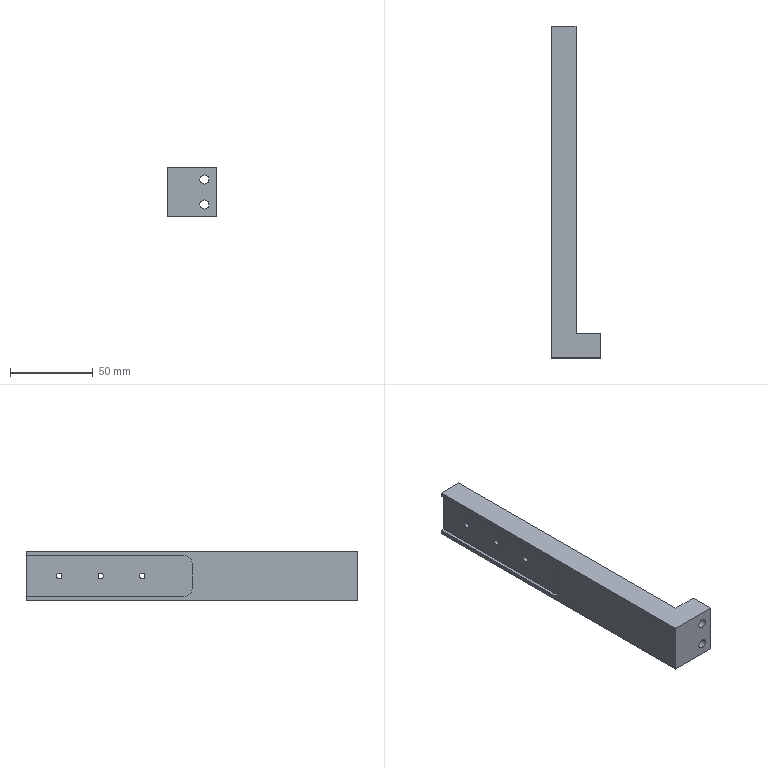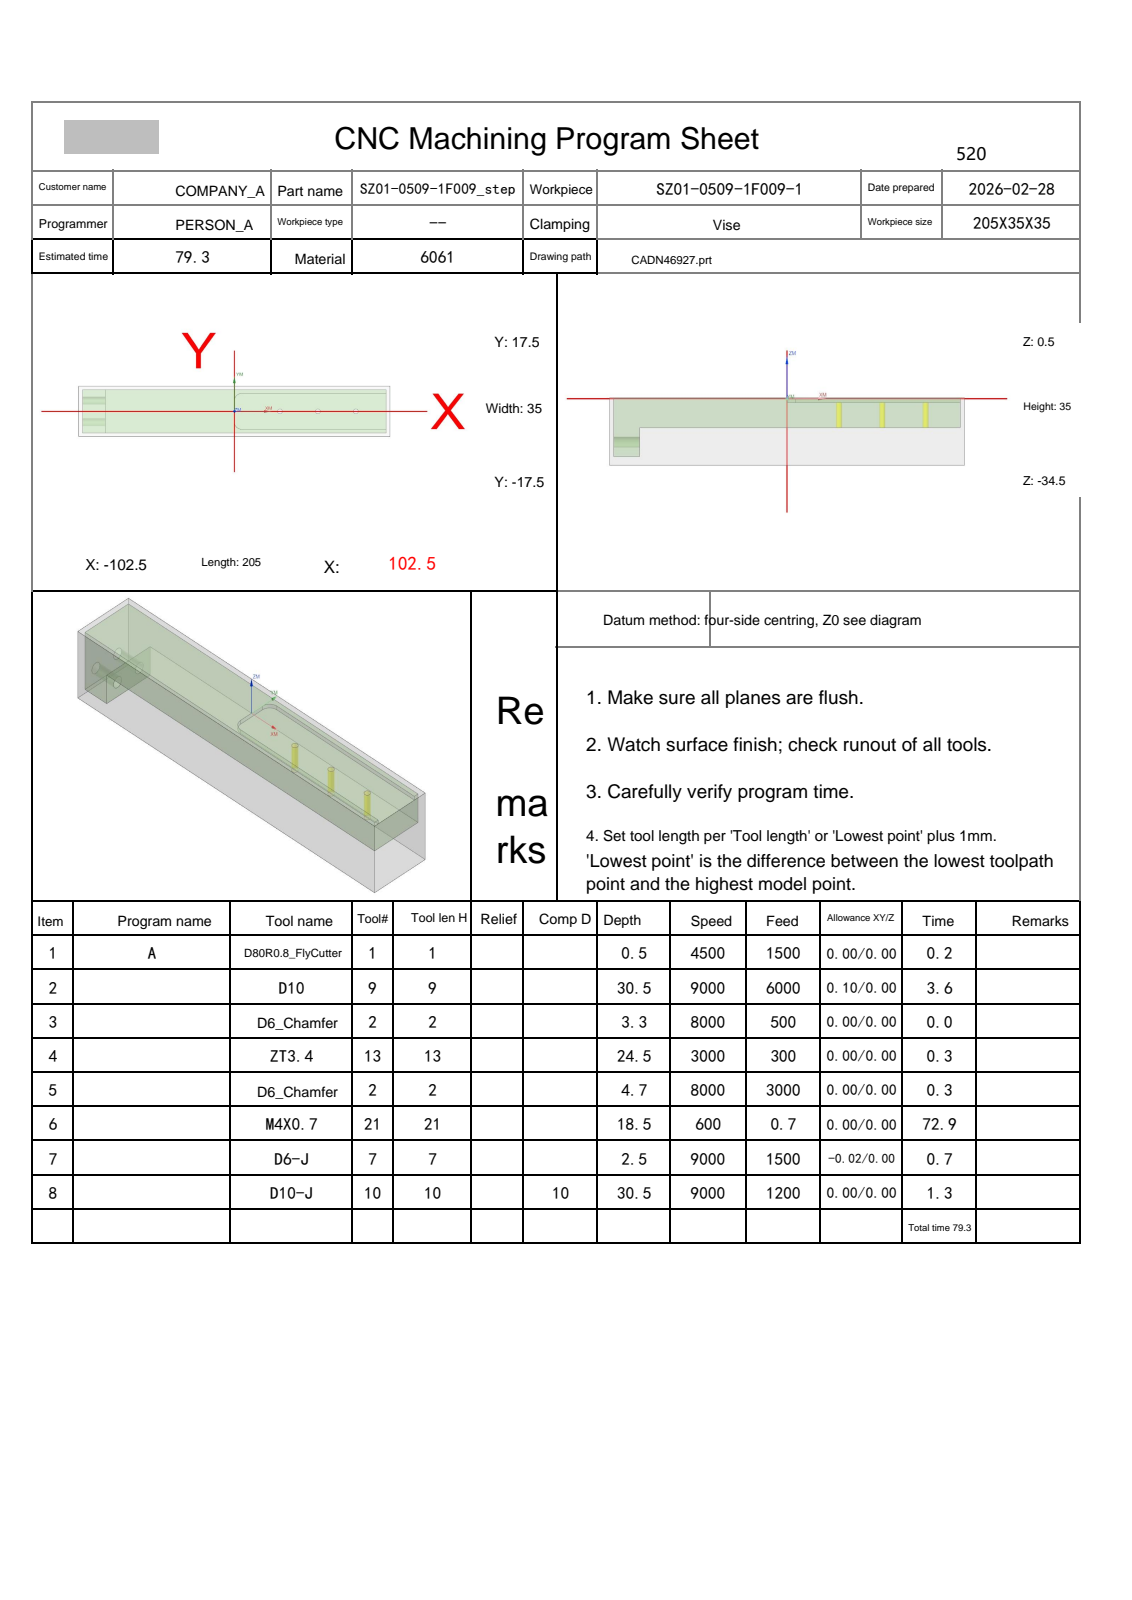NC program | NX | posted by the shop | part box 30 x 200 x 30 mm
Whole program:
%
O0001
(Machine time: 149.40 MIN)
(===Total Tool:7===)
(T1=D80R0.8-FlyCutter D=80.  R=0.8  D-  H01 Z=0.    )
(T9=D10     D=10.  R=0.   D-  H09 Z=-30.  )
(T2=D6_Chamfer   D=6.   R=0.   D-  H02 Z=-4.2  )
(T13=ZT3.4  D=3.4  DR_a=118 D-  H13 Z=-24.  )
(T21=M4X0.7 D=3.3  DR_a=180 D-  H21 Z=-18.  )
(T7=D6-J    D=6.   R=0.   D7  H07 Z=-2.   )
(T10=D10-J  D=10.  R=0.   D10 H10 Z=-30.  )
G80 G90 G17 G49 G40
G91 G28 Z0
M01
N1 T01 M06
(D80R0.8-FlyCutter  D=80. R=0.8 H=01 ce=0.00 di=0.00)
G00 G90 G54 X-145. Y0.0 M03 S4500
G43 H01 Z50.
M08
Z2.
G01 Z0.0 F1500.
X-140.
X140.
X145.
Z2.
G00 Z50.
G91 G28 Z0.0
M05
M09
G91 G28 Z0.0
M01
N2 T09 M06
(D10  D=10. R=0. H=09 ce=0.10 di=0.00)
G00 G90 G54 X0.0 Y20.1 M03 S8000
G43 H09 Z50.
M08
Z.5
G01 X100. Z.341 F6000.
G02 X105.1 Y15. Z.328 I0.0 J-5.1
G01 Y-15. Z.281
G02 X100. Y-20.1 Z.268 I-5.1 J0.0
G01 X-100. Z-.05
G02 X-105.1 Y-15. Z-.063 I0.0 J5.1
G01 Y15. Z-.11
G02 X-100. Y20.1 Z-.123 I5.1 J0.0
G01 X100. Z-.441
G02 X105.1 Y15. Z-.454 I0.0 J-5.1
G01 Y-15. Z-.501
G02 X100. Y-20.1 Z-.514 I-5.1 J0.0
G01 X-100. Z-.832
G02 X-105.1 Y-15. Z-.845 I0.0 J5.1
G01 Y15. Z-.892
G02 X-100. Y20.1 Z-.905 I5.1 J0.0
G01 X100. Z-1.223
G02 X105.1 Y15. Z-1.236 I0.0 J-5.1
G01 Y-15. Z-1.283
G02 X100. Y-20.1 Z-1.296 I-5.1 J0.0
G01 X-100. Z-1.614
G02 X-105.1 Y-15. Z-1.627 I0.0 J5.1
G01 Y15. Z-1.674
G02 X-100. Y20.1 Z-1.687 I5.1 J0.0
G01 X100. Z-2.005
G02 X105.1 Y15. Z-2.018 I0.0 J-5.1
G01 Y-15. Z-2.066
G02 X100. Y-20.1 Z-2.078 I-5.1 J0.0
G01 X-100. Z-2.396
G02 X-105.1 Y-15. Z-2.409 I0.0 J5.1
G01 Y15. Z-2.457
G02 X-100. Y20.1 Z-2.469 I5.1 J0.0
G01 X100. Z-2.787
G02 X105.1 Y15. Z-2.8 I0.0 J-5.1
G01 Y-15. Z-2.848
G02 X100. Y-20.1 Z-2.86 I-5.1 J0.0
G01 X-100. Z-3.178
G02 X-105.1 Y-15. Z-3.191 I0.0 J5.1
G01 Y15. Z-3.239
G02 X-100. Y20.1 Z-3.251 I5.1 J0.0
G01 X100. Z-3.569
G02 X105.1 Y15. Z-3.582 I0.0 J-5.1
G01 Y-15. Z-3.63
G02 X100. Y-20.1 Z-3.642 I-5.1 J0.0
G01 X-100. Z-3.96
G02 X-105.1 Y-15. Z-3.973 I0.0 J5.1
G01 Y15. Z-4.021
G02 X-100. Y20.1 Z-4.033 I5.1 J0.0
G01 X100. Z-4.351
G02 X105.1 Y15. Z-4.364 I0.0 J-5.1
G01 Y-15. Z-4.412
G02 X100. Y-20.1 Z-4.424 I-5.1 J0.0
G01 X-100. Z-4.742
G02 X-105.1 Y-15. Z-4.755 I0.0 J5.1
G01 Y15. Z-4.803
G02 X-100. Y20.1 Z-4.815 I5.1 J0.0
G01 X100. Z-5.133
G02 X105.1 Y15. Z-5.146 I0.0 J-5.1
G01 Y-15. Z-5.194
G02 X100. Y-20.1 Z-5.206 I-5.1 J0.0
G01 X-100. Z-5.524
G02 X-105.1 Y-15. Z-5.537 I0.0 J5.1
G01 Y15. Z-5.585
G02 X-100. Y20.1 Z-5.597 I5.1 J0.0
G01 X100. Z-5.915
G02 X105.1 Y15. Z-5.928 I0.0 J-5.1
G01 Y-15. Z-5.976
G02 X100. Y-20.1 Z-5.988 I-5.1 J0.0
G01 X-100. Z-6.306
G02 X-105.1 Y-15. Z-6.319 I0.0 J5.1
G01 Y15. Z-6.367
G02 X-100. Y20.1 Z-6.38 I5.1 J0.0
G01 X100. Z-6.697
G02 X105.1 Y15. Z-6.71 I0.0 J-5.1
G01 Y-15. Z-6.758
G02 X100. Y-20.1 Z-6.771 I-5.1 J0.0
G01 X-100. Z-7.088
G02 X-105.1 Y-15. Z-7.101 I0.0 J5.1
G01 Y15. Z-7.149
G02 X-100. Y20.1 Z-7.162 I5.1 J0.0
G01 X100. Z-7.479
G02 X105.1 Y15. Z-7.492 I0.0 J-5.1
G01 Y-15. Z-7.54
G02 X100. Y-20.1 Z-7.553 I-5.1 J0.0
G01 X-100. Z-7.87
G02 X-105.1 Y-15. Z-7.883 I0.0 J5.1
G01 Y15. Z-7.931
G02 X-100. Y20.1 Z-7.944 I5.1 J0.0
G01 X100. Z-8.262
G02 X105.1 Y15. Z-8.274 I0.0 J-5.1
G01 Y-15. Z-8.322
G02 X100. Y-20.1 Z-8.335 I-5.1 J0.0
G01 X-100. Z-8.653
G02 X-105.1 Y-15. Z-8.665 I0.0 J5.1
G01 Y15. Z-8.713
G02 X-100. Y20.1 Z-8.726 I5.1 J0.0
G01 X100. Z-9.044
G02 X105.1 Y15. Z-9.056 I0.0 J-5.1
G01 Y-15. Z-9.104
G02 X100. Y-20.1 Z-9.117 I-5.1 J0.0
G01 X-100. Z-9.435
G02 X-105.1 Y-15. Z-9.447 I0.0 J5.1
G01 Y15. Z-9.495
G02 X-100. Y20.1 Z-9.508 I5.1 J0.0
G01 X100. Z-9.826
G02 X105.1 Y15. Z-9.838 I0.0 J-5.1
G01 Y-15. Z-9.886
G02 X100. Y-20.1 Z-9.899 I-5.1 J0.0
G01 X-100. Z-10.217
G02 X-105.1 Y-15. Z-10.229 I0.0 J5.1
G01 Y15. Z-10.277
G02 X-100. Y20.1 Z-10.29 I5.1 J0.0
G01 X100. Z-10.608
G02 X105.1 Y15. Z-10.62 I0.0 J-5.1
G01 Y-15. Z-10.668
G02 X100. Y-20.1 Z-10.681 I-5.1 J0.0
G01 X-100. Z-10.999
G02 X-105.1 Y-15. Z-11.011 I0.0 J5.1
G01 Y15. Z-11.059
G02 X-100. Y20.1 Z-11.072 I5.1 J0.0
G01 X100. Z-11.39
G02 X105.1 Y15. Z-11.402 I0.0 J-5.1
G01 Y-15. Z-11.45
G02 X100. Y-20.1 Z-11.463 I-5.1 J0.0
G01 X-100. Z-11.781
G02 X-105.1 Y-15. Z-11.793 I0.0 J5.1
G01 Y15. Z-11.841
G02 X-100. Y20.1 Z-11.854 I5.1 J0.0
G01 X100. Z-12.172
G02 X105.1 Y15. Z-12.184 I0.0 J-5.1
G01 Y-15. Z-12.232
G02 X100. Y-20.1 Z-12.245 I-5.1 J0.0
G01 X-100. Z-12.563
G02 X-105.1 Y-15. Z-12.576 I0.0 J5.1
G01 Y15. Z-12.623
G02 X-100. Y20.1 Z-12.636 I5.1 J0.0
G01 X100. Z-12.954
G02 X105.1 Y15. Z-12.967 I0.0 J-5.1
G01 Y-15. Z-13.014
G02 X100. Y-20.1 Z-13.027 I-5.1 J0.0
G01 X-100. Z-13.345
G02 X-105.1 Y-15. Z-13.358 I0.0 J5.1
G01 Y15. Z-13.405
G02 X-100. Y20.1 Z-13.418 I5.1 J0.0
G01 X100. Z-13.736
G02 X105.1 Y15. Z-13.749 I0.0 J-5.1
G01 Y-15. Z-13.796
G02 X100. Y-20.1 Z-13.809 I-5.1 J0.0
G01 X-100. Z-14.127
G02 X-105.1 Y-15. Z-14.14 I0.0 J5.1
G01 Y15. Z-14.187
G02 X-100. Y20.1 Z-14.2 I5.1 J0.0
G01 X100. Z-14.518
G02 X105.1 Y15. Z-14.531 I0.0 J-5.1
G01 Y-15. Z-14.578
G02 X100. Y-20.1 Z-14.591 I-5.1 J0.0
G01 X-100. Z-14.909
G02 X-105.1 Y-15. Z-14.922 I0.0 J5.1
G01 Y15. Z-14.969
G02 X-100. Y20.1 Z-14.982 I5.1 J0.0
G01 X100. Z-15.3
G02 X105.1 Y15. Z-15.313 I0.0 J-5.1
G01 Y-15. Z-15.36
G02 X100. Y-20.1 Z-15.373 I-5.1 J0.0
G01 X-100. Z-15.691
G02 X-105.1 Y-15. Z-15.704 I0.0 J5.1
G01 Y15. Z-15.751
G02 X-100. Y20.1 Z-15.764 I5.1 J0.0
G01 X100. Z-16.082
G02 X105.1 Y15. Z-16.095 I0.0 J-5.1
G01 Y-15. Z-16.142
G02 X100. Y-20.1 Z-16.155 I-5.1 J0.0
G01 X-100. Z-16.473
G02 X-105.1 Y-15. Z-16.486 I0.0 J5.1
G01 Y15. Z-16.533
G02 X-100. Y20.1 Z-16.546 I5.1 J0.0
G01 X100. Z-16.864
G02 X105.1 Y15. Z-16.877 I0.0 J-5.1
G01 Y-15. Z-16.924
G02 X100. Y-20.1 Z-16.937 I-5.1 J0.0
G01 X-100. Z-17.255
G02 X-105.1 Y-15. Z-17.268 I0.0 J5.1
G01 Y15. Z-17.316
G02 X-100. Y20.1 Z-17.328 I5.1 J0.0
G01 X100. Z-17.646
G02 X105.1 Y15. Z-17.659 I0.0 J-5.1
G01 Y-15. Z-17.707
G02 X100. Y-20.1 Z-17.719 I-5.1 J0.0
G01 X-100. Z-18.037
G02 X-105.1 Y-15. Z-18.05 I0.0 J5.1
G01 Y15. Z-18.098
G02 X-100. Y20.1 Z-18.11 I5.1 J0.0
G01 X100. Z-18.428
G02 X105.1 Y15. Z-18.441 I0.0 J-5.1
G01 Y-15. Z-18.489
G02 X100. Y-20.1 Z-18.501 I-5.1 J0.0
G01 X-100. Z-18.819
G02 X-105.1 Y-15. Z-18.832 I0.0 J5.1
G01 Y15. Z-18.88
G02 X-100. Y20.1 Z-18.892 I5.1 J0.0
G01 X100. Z-19.21
G02 X105.1 Y15. Z-19.223 I0.0 J-5.1
G01 Y-15. Z-19.271
G02 X100. Y-20.1 Z-19.283 I-5.1 J0.0
G01 X-100. Z-19.601
G02 X-105.1 Y-15. Z-19.614 I0.0 J5.1
G01 Y15. Z-19.662
G02 X-100. Y20.1 Z-19.674 I5.1 J0.0
G01 X100. Z-19.992
G02 X105.1 Y15. Z-20.005 I0.0 J-5.1
G01 Y-15. Z-20.053
G02 X100. Y-20.1 Z-20.065 I-5.1 J0.0
G01 X-100. Z-20.383
G02 X-105.1 Y-15. Z-20.396 I0.0 J5.1
G01 Y15. Z-20.444
G02 X-100. Y20.1 Z-20.456 I5.1 J0.0
G01 X100. Z-20.774
G02 X105.1 Y15. Z-20.787 I0.0 J-5.1
G01 Y-15. Z-20.835
G02 X100. Y-20.1 Z-20.847 I-5.1 J0.0
G01 X-100. Z-21.165
G02 X-105.1 Y-15. Z-21.178 I0.0 J5.1
G01 Y15. Z-21.226
G02 X-100. Y20.1 Z-21.238 I5.1 J0.0
G01 X100. Z-21.556
G02 X105.1 Y15. Z-21.569 I0.0 J-5.1
G01 Y-15. Z-21.617
G02 X100. Y-20.1 Z-21.63 I-5.1 J0.0
G01 X-100. Z-21.947
G02 X-105.1 Y-15. Z-21.96 I0.0 J5.1
G01 Y15. Z-22.008
G02 X-100. Y20.1 Z-22.021 I5.1 J0.0
G01 X100. Z-22.338
G02 X105.1 Y15. Z-22.351 I0.0 J-5.1
G01 Y-15. Z-22.399
G02 X100. Y-20.1 Z-22.412 I-5.1 J0.0
G01 X-100. Z-22.729
G02 X-105.1 Y-15. Z-22.742 I0.0 J5.1
G01 Y15. Z-22.79
G02 X-100. Y20.1 Z-22.803 I5.1 J0.0
G01 X100. Z-23.12
G02 X105.1 Y15. Z-23.133 I0.0 J-5.1
G01 Y-15. Z-23.181
G02 X100. Y-20.1 Z-23.194 I-5.1 J0.0
G01 X-100. Z-23.512
G02 X-105.1 Y-15. Z-23.524 I0.0 J5.1
G01 Y15. Z-23.572
G02 X-100. Y20.1 Z-23.585 I5.1 J0.0
G01 X100. Z-23.903
G02 X105.1 Y15. Z-23.915 I0.0 J-5.1
G01 Y-15. Z-23.963
G02 X100. Y-20.1 Z-23.976 I-5.1 J0.0
G01 X-100. Z-24.294
G02 X-105.1 Y-15. Z-24.306 I0.0 J5.1
G01 Y15. Z-24.354
G02 X-100. Y20.1 Z-24.367 I5.1 J0.0
G01 X100. Z-24.685
G02 X105.1 Y15. Z-24.697 I0.0 J-5.1
G01 Y-15. Z-24.745
G02 X100. Y-20.1 Z-24.758 I-5.1 J0.0
G01 X-100. Z-25.076
G02 X-105.1 Y-15. Z-25.088 I0.0 J5.1
G01 Y15. Z-25.136
G02 X-100. Y20.1 Z-25.149 I5.1 J0.0
G01 X100. Z-25.467
G02 X105.1 Y15. Z-25.479 I0.0 J-5.1
G01 Y-15. Z-25.527
G02 X100. Y-20.1 Z-25.54 I-5.1 J0.0
G01 X-100. Z-25.858
G02 X-105.1 Y-15. Z-25.87 I0.0 J5.1
G01 Y15. Z-25.918
G02 X-100. Y20.1 Z-25.931 I5.1 J0.0
G01 X100. Z-26.249
G02 X105.1 Y15. Z-26.261 I0.0 J-5.1
G01 Y-15. Z-26.309
G02 X100. Y-20.1 Z-26.322 I-5.1 J0.0
G01 X-100. Z-26.64
G02 X-105.1 Y-15. Z-26.652 I0.0 J5.1
G01 Y15. Z-26.7
G02 X-100. Y20.1 Z-26.713 I5.1 J0.0
G01 X100. Z-27.031
G02 X105.1 Y15. Z-27.043 I0.0 J-5.1
G01 Y-15. Z-27.091
G02 X100. Y-20.1 Z-27.104 I-5.1 J0.0
G01 X-100. Z-27.422
G02 X-105.1 Y-15. Z-27.434 I0.0 J5.1
G01 Y15. Z-27.482
G02 X-100. Y20.1 Z-27.495 I5.1 J0.0
G01 X100. Z-27.813
G02 X105.1 Y15. Z-27.826 I0.0 J-5.1
G01 Y-15. Z-27.873
G02 X100. Y-20.1 Z-27.886 I-5.1 J0.0
G01 X-100. Z-28.204
G02 X-105.1 Y-15. Z-28.217 I0.0 J5.1
G01 Y15. Z-28.264
G02 X-100. Y20.1 Z-28.277 I5.1 J0.0
G01 X100. Z-28.595
G02 X105.1 Y15. Z-28.608 I0.0 J-5.1
G01 Y-15. Z-28.655
G02 X100. Y-20.1 Z-28.668 I-5.1 J0.0
G01 X-100. Z-28.986
G02 X-105.1 Y-15. Z-28.999 I0.0 J5.1
G01 Y15. Z-29.046
G02 X-100. Y20.1 Z-29.059 I5.1 J0.0
G01 X100. Z-29.377
G02 X105.1 Y15. Z-29.39 I0.0 J-5.1
G01 Y-15. Z-29.437
G02 X100. Y-20.1 Z-29.45 I-5.1 J0.0
G01 X-100. Z-29.768
G02 X-105.1 Y-15. Z-29.781 I0.0 J5.1
G01 Y15. Z-29.828
G02 X-100. Y20.1 Z-29.841 I5.1 J0.0
G01 X0.0 Z-30.
X100.
G02 X105.1 Y15. I0.0 J-5.1
G01 Y-15.
G02 X100. Y-20.1 I-5.1 J0.0
G01 X-100.
G02 X-105.1 Y-15. I0.0 J5.1
G01 Y15.
G02 X-100. Y20.1 I5.1 J0.0
G01 X0.0
X.5
Z-29.
G00 Z50.
G00 G90 X103.02 Y0.0 M03 S9000
Z50.
Z.52
G01 Z.02 F6000.
X100.02
Y-.402
Y-7.402
X5.098
Y7.402
X100.02
Y.402
Y0.0
X93.02
Y-.402
X12.098
Y.402
X93.02
Y0.0
Z1.02
G00 Z1.5
X103.02
Z.04
G01 Z-.46
X100.02
Y-.4
Y-7.4
X93.02
X5.1
Y7.4
X100.02
Y.4
Y0.0
X93.02
Y-.4
X12.1
Y.4
X93.02
Y0.0
Z.54
G00 Z1.02
X103.02
Z-.44
G01 Z-.94
X100.02
Y-.4
Y-7.4
X93.02
X5.1
Y7.4
X100.02
Y.4
Y0.0
X93.02
Y-.4
X12.1
Y.4
X93.02
Y0.0
Z.06
G00 Z.54
X103.02
Z-.92
G01 Z-1.42
X100.02
Y-.4
Y-7.4
X93.02
X5.1
Y7.4
X100.02
Y.4
Y0.0
X93.02
Y-.4
X12.1
Y.4
X93.02
Y0.0
Z-.42
G00 Z.06
X103.02
Z-1.4
G01 Z-1.9
X100.02
Y-.4
Y-7.4
X93.02
X5.1
Y7.4
X100.02
Y.4
Y0.0
X93.02
Y-.4
X12.1
Y.4
X93.02
Y0.0
Z-.9
G00 Z50.
G91 G28 Z0.0
M05
M09
G91 G28 Z0.0
M01
N3 T02 M06
(D6_Chamfer  D=6. R=0. H=02 ce=0.00 di=0.10)
G00 G90 G54 X30. Y0.0 M03 S8000
G43 H02 Z50.
M08
G98 G81 X30. Y0.0 Z-2.8 R-1. F500.
X55.
X80.
G80
G00 Z50.
G91 G28 Z0.0
M05
M09
G91 G28 Z0.0
M01
N4 T13 M06
(ZT3.4 D=3.4 DR_a=118 H=13)
G00 G90 G54 X30. Y0.0 M03 S3000
G43 H13 Z50.
M08
G98 G83 X30. Y0.0 Z-24. R-1. F300. Q2.
X55.
X80.
G80
G00 Z50.
G91 G28 Z0.0
M05
M09
G91 G28 Z0.0
M01
N5 T02 M06
(D6_Chamfer  D=6. R=0. H=02 ce=0.00 di=0.00)
G00 G90 G54 X.25 Y-17.128 M03 S8000
G43 H02 Z50.
M08
Z2.099
G01 Z-1.5 F3000.
G03 X.33 Y-16.828 I-.52 J.3
X.03 Y-16.308 I-.6 J0.0
G01 X0.0 Y-16.3
X-100.
G02 X-101.3 Y-15. I0.0 J1.3
G01 Y15.
G02 X-100. Y16.3 I1.3 J0.0
G01 X100.
G02 X101.3 Y15. I0.0 J-1.3
G01 Y12.5
G02 X100. Y11.2 I-1.3 J0.0
G01 X5.
G03 X1.3 Y7.5 I0.0 J-3.7
G01 Y-7.5
G03 X5. Y-11.2 I3.7 J0.0
G01 X100.
G02 X101.3 Y-12.5 I0.0 J-1.3
G01 Y-15.
G02 X100. Y-16.3 I-1.3 J0.0
G01 X0.0
X-.03 Y-16.308
G03 X-.33 Y-16.828 I.3 J-.52
X-.25 Y-17.128 I.6 J0.0
G01 Z2.099
G00 Z50.
X102.128 Y9.478
Z1.755
G01 Z-3.499
G03 X101.828 Y9.559 I-.3 J-.52
X101.308 Y9.259 I0.0 J-.6
G01 X101.3 Y9.229
Y-9.229
X101.308 Y-9.259
G03 X101.828 Y-9.559 I.52 J.3
X102.128 Y-9.478 I0.0 J.6
G01 Z1.755
G00 Z50.
G00 G90 X30. Y0.0 M03 S8000
Z50.
G98 G81 X30. Y0.0 Z-4.2 R1. F500.
X55.
X80.
G80
G00 Z50.
G91 G28 Z0.0
M05
M09
G91 G28 Z0.0
M01
N6 T21 M06
(M4X0.7 D=3.3 DR_a=180 H=21)
G00 G90 G54 X30. Y0.0 M03 S600
G43 H21 Z50.
M08
G95
G98 G84 X30. Y0.0 Z-18. R-1. F.7 Q4.
X55.
X80.
G80
G94
G00 Z50.
G91 G28 Z0.0
M05
M09
G91 G28 Z0.0
M01
N7 T07 M06
(D6-J  D=6. R=0. H=07 ce=0.30 di=0.00)
G00 G90 G54 X106. Y0.0 M03 S9000
G43 H07 Z50.
M08
Z-1.5
G01 Z-2. F1500.
X100.6
Y-9.2
X5.
G02 X3.3 Y-7.5 I0.0 J1.7
G01 Y7.5
G02 X5. Y9.2 I1.7 J0.0
G01 X100.6
Y0.0
X96.4
Y-5.
X7.5
Y5.
X96.4
Y0.0
X92.2
Y-.8
X11.7
Y.8
X92.2
Y0.0
Y-.5
X106.
Z-1.5
G00 Z50.
G00 G90 X103.7 Y8.42 M03 S9000
Z50.
Z-1.495
G01 Z-1.995 F1000.
G41 D07
Y8.52
G03 X102.7 Y9.52 I-1. J0.0
G01 X5.
G03 X2.98 Y7.5 I0.0 J-2.02
G01 Y-7.5
G03 X5. Y-9.52 I2.02 J0.0
G01 X102.7
G03 X103.7 Y-8.52 I0.0 J1.
G01 G40 Y-8.42
Z-1.495
G00 Z50.
G91 G28 Z0.0
M05
M09
G91 G28 Z0.0
M01
N8 T10 M06
(D10-J  D=10. R=0. H=10 ce=0.00 di=0.00)
G00 G90 G54 X101.013 Y-21.116 M03 S9000
G43 H10 Z50.
M08
Z-9.5
G01 Z-10. F1200.
G41 D10
X100.997 Y-20.917
G03 X100. Y-20. I-.997 J-.083
G01 X-100.
G02 X-105. Y-15. I0.0 J5.
G01 Y15.
G02 X-100. Y20. I5. J0.0
G01 X100.
G02 X105. Y15. I0.0 J-5.
G01 Y-15.
G02 X100. Y-20. I-5. J0.0
G01 X99.5
G03 X98.5 Y-21. I0.0 J-1.
G01 G40 Y-21.2
Z-9.5
G00 Z50.
X101.013 Y-21.116
Z-19.5
G01 Z-20.
G41 D10
X100.997 Y-20.917
G03 X100. Y-20. I-.997 J-.083
G01 X-100.
G02 X-105. Y-15. I0.0 J5.
G01 Y15.
G02 X-100. Y20. I5. J0.0
G01 X100.
G02 X105. Y15. I0.0 J-5.
G01 Y-15.
G02 X100. Y-20. I-5. J0.0
G01 X99.5
G03 X98.5 Y-21. I0.0 J-1.
G01 G40 Y-21.2
Z-19.5
G00 Z50.
X101.013 Y-21.116
Z-29.5
G01 Z-30.
G41 D10
X100.997 Y-20.917
G03 X100. Y-20. I-.997 J-.083
G01 X-100.
G02 X-105. Y-15. I0.0 J5.
G01 Y15.
G02 X-100. Y20. I5. J0.0
G01 X100.
G02 X105. Y15. I0.0 J-5.
G01 Y-15.
G02 X100. Y-20. I-5. J0.0
G01 X99.5
G03 X98.5 Y-21. I0.0 J-1.
G01 G40 Y-21.2
Z-29.5
G00 Z50.
M05
M09
G91 G28 Z0.0
G91 G28 Y0.0
M30
%